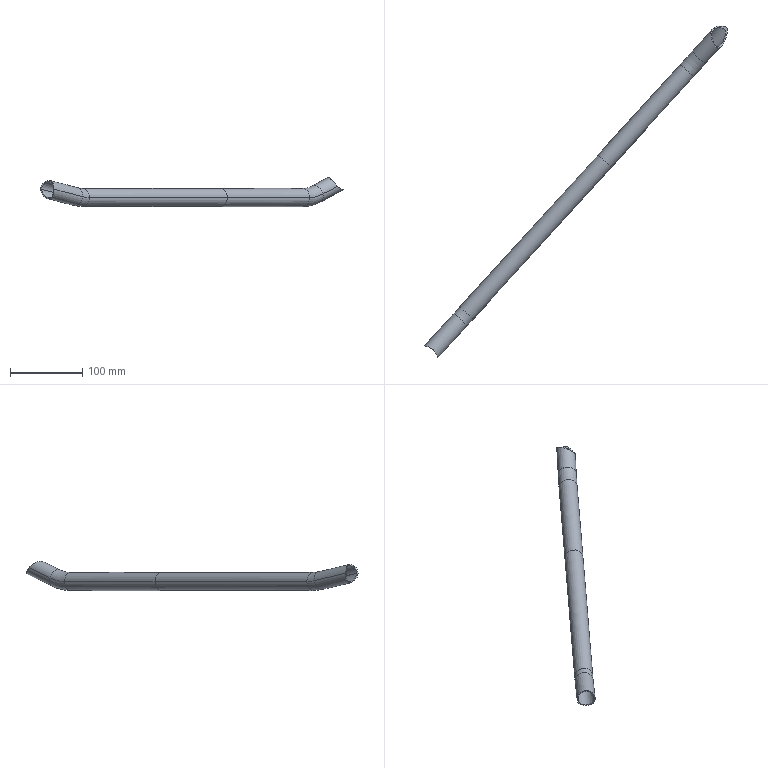Part | STEP file | PRT0001_68_9 | 1 solid | 26 faces | box 418.507 x 458.308 x 40.27 mm | volume 65357 mm3 | cylinder 18 | torus 8 | commonest cylinder face diameters 22 x8 25 x8 43 x1 50 x1